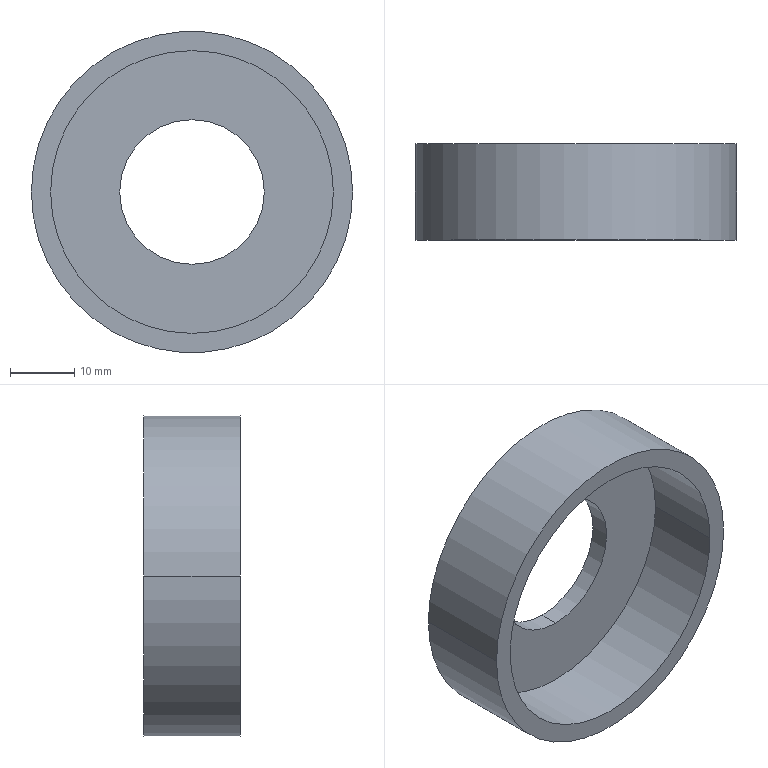Part | NX | 1 solid | 9 faces | box 50 x 15 x 50 mm | volume 10013 mm3 | cylinder 6 | plane 3 | commonest cylinder face diameters 22.5 x2 44 x2 50 x2
STEP:
#1=CARTESIAN_POINT('',(25.,0.,0.));
#2=VERTEX_POINT('',#1);
#3=CARTESIAN_POINT('',(-25.,0.,0.));
#4=VERTEX_POINT('',#3);
#5=CARTESIAN_POINT('',(0.,0.,0.));
#6=DIRECTION('',(0.,-1.,0.));
#7=DIRECTION('',(-1.,0.,0.));
#8=AXIS2_PLACEMENT_3D('',#5,#6,#7);
#9=CIRCLE('',#8,25.);
#10=EDGE_CURVE('',#2,#4,#9,.T.);
#11=ORIENTED_EDGE('',*,*,#10,.F.);
#12=CARTESIAN_POINT('',(0.,0.,0.));
#13=DIRECTION('',(0.,-1.,0.));
#14=DIRECTION('',(-1.,0.,0.));
#15=AXIS2_PLACEMENT_3D('',#12,#13,#14);
#16=CIRCLE('',#15,25.);
#17=EDGE_CURVE('',#4,#2,#16,.T.);
#18=ORIENTED_EDGE('',*,*,#17,.F.);
#19=EDGE_LOOP('',(#11,#18));
#20=FACE_BOUND('',#19,.T.);
#21=CARTESIAN_POINT('',(0.,0.,11.25));
#22=VERTEX_POINT('',#21);
#23=CARTESIAN_POINT('',(0.,0.,-11.25));
#24=VERTEX_POINT('',#23);
#25=CARTESIAN_POINT('',(0.,0.,0.));
#26=DIRECTION('',(0.,1.,0.));
#27=DIRECTION('',(0.,0.,-1.));
#28=AXIS2_PLACEMENT_3D('',#25,#26,#27);
#29=CIRCLE('',#28,11.25);
#30=EDGE_CURVE('',#22,#24,#29,.T.);
#31=ORIENTED_EDGE('',*,*,#30,.F.);
#32=CARTESIAN_POINT('',(0.,0.,0.));
#33=DIRECTION('',(0.,1.,0.));
#34=DIRECTION('',(0.,0.,-1.));
#35=AXIS2_PLACEMENT_3D('',#32,#33,#34);
#36=CIRCLE('',#35,11.25);
#37=EDGE_CURVE('',#24,#22,#36,.T.);
#38=ORIENTED_EDGE('',*,*,#37,.F.);
#39=EDGE_LOOP('',(#31,#38));
#40=FACE_BOUND('',#39,.T.);
#41=CARTESIAN_POINT('',(0.,0.,0.));
#42=DIRECTION('',(0.,-1.,0.));
#43=DIRECTION('',(0.,0.,-1.));
#44=AXIS2_PLACEMENT_3D('',#41,#42,#43);
#45=PLANE('',#44);
#46=ADVANCED_FACE('',(#20,#40),#45,.F.);
#47=CARTESIAN_POINT('',(-25.,-15.,0.));
#48=VERTEX_POINT('',#47);
#49=CARTESIAN_POINT('',(25.,-15.,0.));
#50=VERTEX_POINT('',#49);
#51=CARTESIAN_POINT('',(0.,-15.,0.));
#52=DIRECTION('',(0.,1.,0.));
#53=DIRECTION('',(1.,0.,0.));
#54=AXIS2_PLACEMENT_3D('',#51,#52,#53);
#55=CIRCLE('',#54,25.);
#56=EDGE_CURVE('',#48,#50,#55,.T.);
#57=ORIENTED_EDGE('',*,*,#56,.T.);
#58=CARTESIAN_POINT('',(25.,0.,0.));
#59=DIRECTION('',(0.,-1.,0.));
#60=VECTOR('',#59,1000.);
#61=LINE('',#58,#60);
#62=EDGE_CURVE('',#2,#50,#61,.T.);
#63=ORIENTED_EDGE('',*,*,#62,.F.);
#64=ORIENTED_EDGE('',*,*,#10,.T.);
#65=CARTESIAN_POINT('',(-25.,0.,0.));
#66=DIRECTION('',(0.,-1.,0.));
#67=VECTOR('',#66,1000.);
#68=LINE('',#65,#67);
#69=EDGE_CURVE('',#4,#48,#68,.T.);
#70=ORIENTED_EDGE('',*,*,#69,.T.);
#71=EDGE_LOOP('',(#57,#63,#64,#70));
#72=FACE_BOUND('',#71,.T.);
#73=CARTESIAN_POINT('',(0.,0.,0.));
#74=DIRECTION('',(0.,-1.,0.));
#75=DIRECTION('',(1.,0.,0.));
#76=AXIS2_PLACEMENT_3D('',#73,#74,#75);
#77=CYLINDRICAL_SURFACE('',#76,25.);
#78=ADVANCED_FACE('',(#72),#77,.T.);
#79=CARTESIAN_POINT('',(22.,-3.,0.));
#80=VERTEX_POINT('',#79);
#81=CARTESIAN_POINT('',(-22.,-3.,0.));
#82=VERTEX_POINT('',#81);
#83=CARTESIAN_POINT('',(0.,-3.,0.));
#84=DIRECTION('',(0.,1.,0.));
#85=DIRECTION('',(-1.,0.,0.));
#86=AXIS2_PLACEMENT_3D('',#83,#84,#85);
#87=CIRCLE('',#86,22.);
#88=EDGE_CURVE('',#80,#82,#87,.T.);
#89=ORIENTED_EDGE('',*,*,#88,.F.);
#90=CARTESIAN_POINT('',(0.,-3.,0.));
#91=DIRECTION('',(0.,1.,0.));
#92=DIRECTION('',(-1.,0.,0.));
#93=AXIS2_PLACEMENT_3D('',#90,#91,#92);
#94=CIRCLE('',#93,22.);
#95=EDGE_CURVE('',#82,#80,#94,.T.);
#96=ORIENTED_EDGE('',*,*,#95,.F.);
#97=EDGE_LOOP('',(#89,#96));
#98=FACE_BOUND('',#97,.T.);
#99=CARTESIAN_POINT('',(0.,-3.,-11.25));
#100=VERTEX_POINT('',#99);
#101=CARTESIAN_POINT('',(0.,-3.,11.25));
#102=VERTEX_POINT('',#101);
#103=CARTESIAN_POINT('',(0.,-3.,0.));
#104=DIRECTION('',(0.,-1.,0.));
#105=DIRECTION('',(0.,0.,1.));
#106=AXIS2_PLACEMENT_3D('',#103,#104,#105);
#107=CIRCLE('',#106,11.25);
#108=EDGE_CURVE('',#100,#102,#107,.T.);
#109=ORIENTED_EDGE('',*,*,#108,.F.);
#110=CARTESIAN_POINT('',(0.,-3.,0.));
#111=DIRECTION('',(0.,-1.,0.));
#112=DIRECTION('',(0.,0.,1.));
#113=AXIS2_PLACEMENT_3D('',#110,#111,#112);
#114=CIRCLE('',#113,11.25);
#115=EDGE_CURVE('',#102,#100,#114,.T.);
#116=ORIENTED_EDGE('',*,*,#115,.F.);
#117=EDGE_LOOP('',(#109,#116));
#118=FACE_BOUND('',#117,.T.);
#119=CARTESIAN_POINT('',(0.,-3.,0.));
#120=DIRECTION('',(0.,-1.,0.));
#121=DIRECTION('',(0.,0.,-1.));
#122=AXIS2_PLACEMENT_3D('',#119,#120,#121);
#123=PLANE('',#122);
#124=ADVANCED_FACE('',(#98,#118),#123,.T.);
#125=ORIENTED_EDGE('',*,*,#56,.F.);
#126=CARTESIAN_POINT('',(0.,-15.,0.));
#127=DIRECTION('',(0.,1.,0.));
#128=DIRECTION('',(1.,0.,0.));
#129=AXIS2_PLACEMENT_3D('',#126,#127,#128);
#130=CIRCLE('',#129,25.);
#131=EDGE_CURVE('',#50,#48,#130,.T.);
#132=ORIENTED_EDGE('',*,*,#131,.F.);
#133=EDGE_LOOP('',(#125,#132));
#134=FACE_BOUND('',#133,.T.);
#135=CARTESIAN_POINT('',(22.,-15.,0.));
#136=VERTEX_POINT('',#135);
#137=CARTESIAN_POINT('',(-22.,-15.,0.));
#138=VERTEX_POINT('',#137);
#139=CARTESIAN_POINT('',(0.,-15.,0.));
#140=DIRECTION('',(0.,-1.,0.));
#141=DIRECTION('',(-1.,0.,0.));
#142=AXIS2_PLACEMENT_3D('',#139,#140,#141);
#143=CIRCLE('',#142,22.);
#144=EDGE_CURVE('',#136,#138,#143,.T.);
#145=ORIENTED_EDGE('',*,*,#144,.F.);
#146=CARTESIAN_POINT('',(0.,-15.,0.));
#147=DIRECTION('',(0.,-1.,0.));
#148=DIRECTION('',(-1.,0.,0.));
#149=AXIS2_PLACEMENT_3D('',#146,#147,#148);
#150=CIRCLE('',#149,22.);
#151=EDGE_CURVE('',#138,#136,#150,.T.);
#152=ORIENTED_EDGE('',*,*,#151,.F.);
#153=EDGE_LOOP('',(#145,#152));
#154=FACE_BOUND('',#153,.T.);
#155=CARTESIAN_POINT('',(0.,-15.,0.));
#156=DIRECTION('',(0.,-1.,0.));
#157=DIRECTION('',(0.,0.,-1.));
#158=AXIS2_PLACEMENT_3D('',#155,#156,#157);
#159=PLANE('',#158);
#160=ADVANCED_FACE('',(#134,#154),#159,.T.);
#161=ORIENTED_EDGE('',*,*,#88,.T.);
#162=CARTESIAN_POINT('',(-22.,0.,0.));
#163=DIRECTION('',(0.,-1.,0.));
#164=VECTOR('',#163,1000.);
#165=LINE('',#162,#164);
#166=EDGE_CURVE('',#138,#82,#165,.F.);
#167=ORIENTED_EDGE('',*,*,#166,.F.);
#168=ORIENTED_EDGE('',*,*,#151,.T.);
#169=CARTESIAN_POINT('',(22.,0.,0.));
#170=DIRECTION('',(0.,-1.,0.));
#171=VECTOR('',#170,1000.);
#172=LINE('',#169,#171);
#173=EDGE_CURVE('',#136,#80,#172,.F.);
#174=ORIENTED_EDGE('',*,*,#173,.T.);
#175=EDGE_LOOP('',(#161,#167,#168,#174));
#176=FACE_BOUND('',#175,.T.);
#177=CARTESIAN_POINT('',(0.,0.,0.));
#178=DIRECTION('',(0.,-1.,0.));
#179=DIRECTION('',(1.,0.,0.));
#180=AXIS2_PLACEMENT_3D('',#177,#178,#179);
#181=CYLINDRICAL_SURFACE('',#180,22.);
#182=ADVANCED_FACE('',(#176),#181,.F.);
#183=ORIENTED_EDGE('',*,*,#108,.T.);
#184=CARTESIAN_POINT('',(0.,-3.,11.25));
#185=DIRECTION('',(0.,-1.,0.));
#186=VECTOR('',#185,1000.);
#187=LINE('',#184,#186);
#188=EDGE_CURVE('',#102,#22,#187,.F.);
#189=ORIENTED_EDGE('',*,*,#188,.T.);
#190=ORIENTED_EDGE('',*,*,#30,.T.);
#191=CARTESIAN_POINT('',(0.,-3.,-11.25));
#192=DIRECTION('',(0.,-1.,0.));
#193=VECTOR('',#192,1000.);
#194=LINE('',#191,#193);
#195=EDGE_CURVE('',#100,#24,#194,.F.);
#196=ORIENTED_EDGE('',*,*,#195,.F.);
#197=EDGE_LOOP('',(#183,#189,#190,#196));
#198=FACE_BOUND('',#197,.T.);
#199=CARTESIAN_POINT('',(0.,-3.,0.));
#200=DIRECTION('',(0.,-1.,0.));
#201=DIRECTION('',(0.,0.,-1.));
#202=AXIS2_PLACEMENT_3D('',#199,#200,#201);
#203=CYLINDRICAL_SURFACE('',#202,11.25);
#204=ADVANCED_FACE('',(#198),#203,.F.);
#205=ORIENTED_EDGE('',*,*,#195,.T.);
#206=ORIENTED_EDGE('',*,*,#37,.T.);
#207=ORIENTED_EDGE('',*,*,#188,.F.);
#208=ORIENTED_EDGE('',*,*,#115,.T.);
#209=EDGE_LOOP('',(#205,#206,#207,#208));
#210=FACE_BOUND('',#209,.T.);
#211=CARTESIAN_POINT('',(0.,-3.,0.));
#212=DIRECTION('',(0.,-1.,0.));
#213=DIRECTION('',(0.,0.,-1.));
#214=AXIS2_PLACEMENT_3D('',#211,#212,#213);
#215=CYLINDRICAL_SURFACE('',#214,11.25);
#216=ADVANCED_FACE('',(#210),#215,.F.);
#217=ORIENTED_EDGE('',*,*,#144,.T.);
#218=ORIENTED_EDGE('',*,*,#166,.T.);
#219=ORIENTED_EDGE('',*,*,#95,.T.);
#220=ORIENTED_EDGE('',*,*,#173,.F.);
#221=EDGE_LOOP('',(#217,#218,#219,#220));
#222=FACE_BOUND('',#221,.T.);
#223=CARTESIAN_POINT('',(0.,0.,0.));
#224=DIRECTION('',(0.,-1.,0.));
#225=DIRECTION('',(1.,0.,0.));
#226=AXIS2_PLACEMENT_3D('',#223,#224,#225);
#227=CYLINDRICAL_SURFACE('',#226,22.);
#228=ADVANCED_FACE('',(#222),#227,.F.);
#229=ORIENTED_EDGE('',*,*,#62,.T.);
#230=ORIENTED_EDGE('',*,*,#131,.T.);
#231=ORIENTED_EDGE('',*,*,#69,.F.);
#232=ORIENTED_EDGE('',*,*,#17,.T.);
#233=EDGE_LOOP('',(#229,#230,#231,#232));
#234=FACE_BOUND('',#233,.T.);
#235=CARTESIAN_POINT('',(0.,0.,0.));
#236=DIRECTION('',(0.,-1.,0.));
#237=DIRECTION('',(1.,0.,0.));
#238=AXIS2_PLACEMENT_3D('',#235,#236,#237);
#239=CYLINDRICAL_SURFACE('',#238,25.);
#240=ADVANCED_FACE('',(#234),#239,.T.);
#241=CLOSED_SHELL('',(#46,#78,#124,#160,#182,#204,#216,#228,#240));
#242=MANIFOLD_SOLID_BREP('',#241);
#243=(LENGTH_UNIT()NAMED_UNIT(*)SI_UNIT(.MILLI.,.METRE.));
#244=UNCERTAINTY_MEASURE_WITH_UNIT(LENGTH_MEASURE(0.00001),#243,'','');
#245=(NAMED_UNIT(*)PLANE_ANGLE_UNIT()SI_UNIT($,.RADIAN.));
#246=(NAMED_UNIT(*)SI_UNIT($,.STERADIAN.)SOLID_ANGLE_UNIT());
#247=(GEOMETRIC_REPRESENTATION_CONTEXT(3)GLOBAL_UNCERTAINTY_ASSIGNED_CONTEXT((#244))GLOBAL_UNIT_ASSIGNED_CONTEXT((#243,#245,#246))REPRESENTATION_CONTEXT('',''));
#248=ADVANCED_BREP_SHAPE_REPRESENTATION('',(#242),#247);